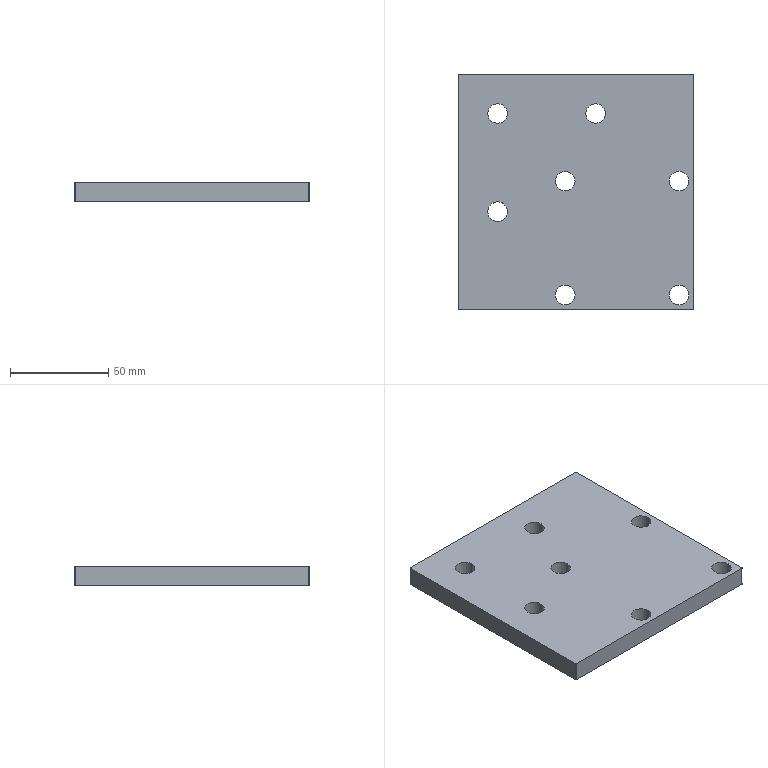Part | STEP file | Pad plate- | 1 solid | 24 faces | box 120 x 120 x 10 mm | volume 138500 mm3 | cylinder 18 | plane 6 | commonest cylinder face diameters 10 x14 1 x4
STEP:
#1=CARTESIAN_POINT('',(-392.5,287.5,10.));
#2=VERTEX_POINT('',#1);
#3=CARTESIAN_POINT('',(-382.5,287.5,10.));
#4=VERTEX_POINT('',#3);
#5=CARTESIAN_POINT('',(-387.5,287.5,10.));
#6=DIRECTION('',(0.,0.,1.));
#7=DIRECTION('',(1.,0.,0.));
#8=AXIS2_PLACEMENT_3D('',#5,#6,#7);
#9=CIRCLE('',#8,5.);
#10=EDGE_CURVE('',#2,#4,#9,.T.);
#11=ORIENTED_EDGE('',*,*,#10,.T.);
#12=CARTESIAN_POINT('',(-382.5,287.5,0.));
#13=VERTEX_POINT('',#12);
#14=CARTESIAN_POINT('',(-382.5,287.5,10.));
#15=DIRECTION('',(0.,0.,-1.));
#16=VECTOR('',#15,1000.);
#17=LINE('',#14,#16);
#18=EDGE_CURVE('',#4,#13,#17,.T.);
#19=ORIENTED_EDGE('',*,*,#18,.T.);
#20=CARTESIAN_POINT('',(-392.5,287.5,0.));
#21=VERTEX_POINT('',#20);
#22=CARTESIAN_POINT('',(-387.5,287.5,0.));
#23=DIRECTION('',(0.,0.,1.));
#24=DIRECTION('',(1.,0.,0.));
#25=AXIS2_PLACEMENT_3D('',#22,#23,#24);
#26=CIRCLE('',#25,5.);
#27=EDGE_CURVE('',#21,#13,#26,.T.);
#28=ORIENTED_EDGE('',*,*,#27,.F.);
#29=CARTESIAN_POINT('',(-392.5,287.5,10.));
#30=DIRECTION('',(0.,0.,-1.));
#31=VECTOR('',#30,1000.);
#32=LINE('',#29,#31);
#33=EDGE_CURVE('',#2,#21,#32,.T.);
#34=ORIENTED_EDGE('',*,*,#33,.F.);
#35=EDGE_LOOP('',(#11,#19,#28,#34));
#36=FACE_OUTER_BOUND('',#35,.T.);
#37=CARTESIAN_POINT('',(-387.5,287.5,10.));
#38=DIRECTION('',(0.,0.,-1.));
#39=DIRECTION('',(-1.,0.,0.));
#40=AXIS2_PLACEMENT_3D('',#37,#38,#39);
#41=CYLINDRICAL_SURFACE('',#40,5.);
#42=ADVANCED_FACE('',(#36),#41,.F.);
#43=CARTESIAN_POINT('',(-450.499,287.494,10.));
#44=VERTEX_POINT('',#43);
#45=CARTESIAN_POINT('',(-440.499,287.494,10.));
#46=VERTEX_POINT('',#45);
#47=CARTESIAN_POINT('',(-445.499,287.494,10.));
#48=DIRECTION('',(0.,0.,1.));
#49=DIRECTION('',(1.,0.,0.));
#50=AXIS2_PLACEMENT_3D('',#47,#48,#49);
#51=CIRCLE('',#50,5.);
#52=EDGE_CURVE('',#44,#46,#51,.T.);
#53=ORIENTED_EDGE('',*,*,#52,.T.);
#54=CARTESIAN_POINT('',(-440.499,287.494,0.));
#55=VERTEX_POINT('',#54);
#56=CARTESIAN_POINT('',(-440.499,287.494,10.));
#57=DIRECTION('',(0.,0.,-1.));
#58=VECTOR('',#57,1000.);
#59=LINE('',#56,#58);
#60=EDGE_CURVE('',#46,#55,#59,.T.);
#61=ORIENTED_EDGE('',*,*,#60,.T.);
#62=CARTESIAN_POINT('',(-450.499,287.494,0.));
#63=VERTEX_POINT('',#62);
#64=CARTESIAN_POINT('',(-445.499,287.494,0.));
#65=DIRECTION('',(0.,0.,1.));
#66=DIRECTION('',(1.,0.,0.));
#67=AXIS2_PLACEMENT_3D('',#64,#65,#66);
#68=CIRCLE('',#67,5.);
#69=EDGE_CURVE('',#63,#55,#68,.T.);
#70=ORIENTED_EDGE('',*,*,#69,.F.);
#71=CARTESIAN_POINT('',(-450.499,287.494,10.));
#72=DIRECTION('',(0.,0.,-1.));
#73=VECTOR('',#72,1000.);
#74=LINE('',#71,#73);
#75=EDGE_CURVE('',#44,#63,#74,.T.);
#76=ORIENTED_EDGE('',*,*,#75,.F.);
#77=EDGE_LOOP('',(#53,#61,#70,#76));
#78=FACE_OUTER_BOUND('',#77,.T.);
#79=CARTESIAN_POINT('',(-445.499,287.494,10.));
#80=DIRECTION('',(0.,0.,-1.));
#81=DIRECTION('',(-1.,0.,0.));
#82=AXIS2_PLACEMENT_3D('',#79,#80,#81);
#83=CYLINDRICAL_SURFACE('',#82,5.);
#84=ADVANCED_FACE('',(#78),#83,.F.);
#85=CARTESIAN_POINT('',(-392.5,345.5,10.));
#86=VERTEX_POINT('',#85);
#87=CARTESIAN_POINT('',(-382.5,345.5,10.));
#88=VERTEX_POINT('',#87);
#89=CARTESIAN_POINT('',(-387.5,345.5,10.));
#90=DIRECTION('',(0.,0.,1.));
#91=DIRECTION('',(1.,0.,0.));
#92=AXIS2_PLACEMENT_3D('',#89,#90,#91);
#93=CIRCLE('',#92,5.);
#94=EDGE_CURVE('',#86,#88,#93,.T.);
#95=ORIENTED_EDGE('',*,*,#94,.T.);
#96=CARTESIAN_POINT('',(-382.5,345.5,0.));
#97=VERTEX_POINT('',#96);
#98=CARTESIAN_POINT('',(-382.5,345.5,10.));
#99=DIRECTION('',(0.,0.,-1.));
#100=VECTOR('',#99,1000.);
#101=LINE('',#98,#100);
#102=EDGE_CURVE('',#88,#97,#101,.T.);
#103=ORIENTED_EDGE('',*,*,#102,.T.);
#104=CARTESIAN_POINT('',(-392.5,345.5,0.));
#105=VERTEX_POINT('',#104);
#106=CARTESIAN_POINT('',(-387.5,345.5,0.));
#107=DIRECTION('',(0.,0.,1.));
#108=DIRECTION('',(1.,0.,0.));
#109=AXIS2_PLACEMENT_3D('',#106,#107,#108);
#110=CIRCLE('',#109,5.);
#111=EDGE_CURVE('',#105,#97,#110,.T.);
#112=ORIENTED_EDGE('',*,*,#111,.F.);
#113=CARTESIAN_POINT('',(-392.5,345.5,10.));
#114=DIRECTION('',(0.,0.,-1.));
#115=VECTOR('',#114,1000.);
#116=LINE('',#113,#115);
#117=EDGE_CURVE('',#86,#105,#116,.T.);
#118=ORIENTED_EDGE('',*,*,#117,.F.);
#119=EDGE_LOOP('',(#95,#103,#112,#118));
#120=FACE_OUTER_BOUND('',#119,.T.);
#121=CARTESIAN_POINT('',(-387.5,345.5,10.));
#122=DIRECTION('',(0.,0.,-1.));
#123=DIRECTION('',(-1.,0.,0.));
#124=AXIS2_PLACEMENT_3D('',#121,#122,#123);
#125=CYLINDRICAL_SURFACE('',#124,5.);
#126=ADVANCED_FACE('',(#120),#125,.F.);
#127=CARTESIAN_POINT('',(-450.494,345.498,10.));
#128=VERTEX_POINT('',#127);
#129=CARTESIAN_POINT('',(-440.494,345.498,10.));
#130=VERTEX_POINT('',#129);
#131=CARTESIAN_POINT('',(-445.494,345.498,10.));
#132=DIRECTION('',(0.,0.,1.));
#133=DIRECTION('',(1.,0.,0.));
#134=AXIS2_PLACEMENT_3D('',#131,#132,#133);
#135=CIRCLE('',#134,5.);
#136=EDGE_CURVE('',#128,#130,#135,.T.);
#137=ORIENTED_EDGE('',*,*,#136,.T.);
#138=CARTESIAN_POINT('',(-440.494,345.498,0.));
#139=VERTEX_POINT('',#138);
#140=CARTESIAN_POINT('',(-440.494,345.498,10.));
#141=DIRECTION('',(0.,0.,-1.));
#142=VECTOR('',#141,1000.);
#143=LINE('',#140,#142);
#144=EDGE_CURVE('',#130,#139,#143,.T.);
#145=ORIENTED_EDGE('',*,*,#144,.T.);
#146=CARTESIAN_POINT('',(-450.494,345.498,0.));
#147=VERTEX_POINT('',#146);
#148=CARTESIAN_POINT('',(-445.494,345.498,0.));
#149=DIRECTION('',(0.,0.,1.));
#150=DIRECTION('',(1.,0.,0.));
#151=AXIS2_PLACEMENT_3D('',#148,#149,#150);
#152=CIRCLE('',#151,5.);
#153=EDGE_CURVE('',#147,#139,#152,.T.);
#154=ORIENTED_EDGE('',*,*,#153,.F.);
#155=CARTESIAN_POINT('',(-450.494,345.498,10.));
#156=DIRECTION('',(0.,0.,-1.));
#157=VECTOR('',#156,1000.);
#158=LINE('',#155,#157);
#159=EDGE_CURVE('',#128,#147,#158,.T.);
#160=ORIENTED_EDGE('',*,*,#159,.F.);
#161=EDGE_LOOP('',(#137,#145,#154,#160));
#162=FACE_OUTER_BOUND('',#161,.T.);
#163=CARTESIAN_POINT('',(-445.494,345.498,10.));
#164=DIRECTION('',(0.,0.,-1.));
#165=DIRECTION('',(-1.,0.,0.));
#166=AXIS2_PLACEMENT_3D('',#163,#164,#165);
#167=CYLINDRICAL_SURFACE('',#166,5.);
#168=ADVANCED_FACE('',(#162),#167,.F.);
#169=CARTESIAN_POINT('',(-485.,330.,10.));
#170=VERTEX_POINT('',#169);
#171=CARTESIAN_POINT('',(-475.,330.,10.));
#172=VERTEX_POINT('',#171);
#173=CARTESIAN_POINT('',(-480.,330.,10.));
#174=DIRECTION('',(0.,0.,1.));
#175=DIRECTION('',(1.,0.,0.));
#176=AXIS2_PLACEMENT_3D('',#173,#174,#175);
#177=CIRCLE('',#176,5.);
#178=EDGE_CURVE('',#170,#172,#177,.T.);
#179=ORIENTED_EDGE('',*,*,#178,.T.);
#180=CARTESIAN_POINT('',(-475.,330.,0.));
#181=VERTEX_POINT('',#180);
#182=CARTESIAN_POINT('',(-475.,330.,10.));
#183=DIRECTION('',(0.,0.,-1.));
#184=VECTOR('',#183,1000.);
#185=LINE('',#182,#184);
#186=EDGE_CURVE('',#172,#181,#185,.T.);
#187=ORIENTED_EDGE('',*,*,#186,.T.);
#188=CARTESIAN_POINT('',(-485.,330.,0.));
#189=VERTEX_POINT('',#188);
#190=CARTESIAN_POINT('',(-480.,330.,0.));
#191=DIRECTION('',(0.,0.,1.));
#192=DIRECTION('',(1.,0.,0.));
#193=AXIS2_PLACEMENT_3D('',#190,#191,#192);
#194=CIRCLE('',#193,5.);
#195=EDGE_CURVE('',#189,#181,#194,.T.);
#196=ORIENTED_EDGE('',*,*,#195,.F.);
#197=CARTESIAN_POINT('',(-485.,330.,10.));
#198=DIRECTION('',(0.,0.,-1.));
#199=VECTOR('',#198,1000.);
#200=LINE('',#197,#199);
#201=EDGE_CURVE('',#170,#189,#200,.T.);
#202=ORIENTED_EDGE('',*,*,#201,.F.);
#203=EDGE_LOOP('',(#179,#187,#196,#202));
#204=FACE_OUTER_BOUND('',#203,.T.);
#205=CARTESIAN_POINT('',(-480.,330.,10.));
#206=DIRECTION('',(0.,0.,-1.));
#207=DIRECTION('',(-1.,0.,0.));
#208=AXIS2_PLACEMENT_3D('',#205,#206,#207);
#209=CYLINDRICAL_SURFACE('',#208,5.);
#210=ADVANCED_FACE('',(#204),#209,.F.);
#211=CARTESIAN_POINT('',(-435.,380.,10.));
#212=VERTEX_POINT('',#211);
#213=CARTESIAN_POINT('',(-425.,380.,10.));
#214=VERTEX_POINT('',#213);
#215=CARTESIAN_POINT('',(-430.,380.,10.));
#216=DIRECTION('',(0.,0.,1.));
#217=DIRECTION('',(1.,0.,0.));
#218=AXIS2_PLACEMENT_3D('',#215,#216,#217);
#219=CIRCLE('',#218,5.);
#220=EDGE_CURVE('',#212,#214,#219,.T.);
#221=ORIENTED_EDGE('',*,*,#220,.T.);
#222=CARTESIAN_POINT('',(-425.,380.,0.));
#223=VERTEX_POINT('',#222);
#224=CARTESIAN_POINT('',(-425.,380.,10.));
#225=DIRECTION('',(0.,0.,-1.));
#226=VECTOR('',#225,1000.);
#227=LINE('',#224,#226);
#228=EDGE_CURVE('',#214,#223,#227,.T.);
#229=ORIENTED_EDGE('',*,*,#228,.T.);
#230=CARTESIAN_POINT('',(-435.,380.,0.));
#231=VERTEX_POINT('',#230);
#232=CARTESIAN_POINT('',(-430.,380.,0.));
#233=DIRECTION('',(0.,0.,1.));
#234=DIRECTION('',(1.,0.,0.));
#235=AXIS2_PLACEMENT_3D('',#232,#233,#234);
#236=CIRCLE('',#235,5.);
#237=EDGE_CURVE('',#231,#223,#236,.T.);
#238=ORIENTED_EDGE('',*,*,#237,.F.);
#239=CARTESIAN_POINT('',(-435.,380.,10.));
#240=DIRECTION('',(0.,0.,-1.));
#241=VECTOR('',#240,1000.);
#242=LINE('',#239,#241);
#243=EDGE_CURVE('',#212,#231,#242,.T.);
#244=ORIENTED_EDGE('',*,*,#243,.F.);
#245=EDGE_LOOP('',(#221,#229,#238,#244));
#246=FACE_OUTER_BOUND('',#245,.T.);
#247=CARTESIAN_POINT('',(-430.,380.,10.));
#248=DIRECTION('',(0.,0.,-1.));
#249=DIRECTION('',(-1.,0.,0.));
#250=AXIS2_PLACEMENT_3D('',#247,#248,#249);
#251=CYLINDRICAL_SURFACE('',#250,5.);
#252=ADVANCED_FACE('',(#246),#251,.F.);
#253=CARTESIAN_POINT('',(-485.,380.,10.));
#254=VERTEX_POINT('',#253);
#255=CARTESIAN_POINT('',(-475.,380.,10.));
#256=VERTEX_POINT('',#255);
#257=CARTESIAN_POINT('',(-480.,380.,10.));
#258=DIRECTION('',(0.,0.,1.));
#259=DIRECTION('',(1.,0.,0.));
#260=AXIS2_PLACEMENT_3D('',#257,#258,#259);
#261=CIRCLE('',#260,5.);
#262=EDGE_CURVE('',#254,#256,#261,.T.);
#263=ORIENTED_EDGE('',*,*,#262,.T.);
#264=CARTESIAN_POINT('',(-475.,380.,0.));
#265=VERTEX_POINT('',#264);
#266=CARTESIAN_POINT('',(-475.,380.,10.));
#267=DIRECTION('',(0.,0.,-1.));
#268=VECTOR('',#267,1000.);
#269=LINE('',#266,#268);
#270=EDGE_CURVE('',#256,#265,#269,.T.);
#271=ORIENTED_EDGE('',*,*,#270,.T.);
#272=CARTESIAN_POINT('',(-485.,380.,0.));
#273=VERTEX_POINT('',#272);
#274=CARTESIAN_POINT('',(-480.,380.,0.));
#275=DIRECTION('',(0.,0.,1.));
#276=DIRECTION('',(1.,0.,0.));
#277=AXIS2_PLACEMENT_3D('',#274,#275,#276);
#278=CIRCLE('',#277,5.);
#279=EDGE_CURVE('',#273,#265,#278,.T.);
#280=ORIENTED_EDGE('',*,*,#279,.F.);
#281=CARTESIAN_POINT('',(-485.,380.,10.));
#282=DIRECTION('',(0.,0.,-1.));
#283=VECTOR('',#282,1000.);
#284=LINE('',#281,#283);
#285=EDGE_CURVE('',#254,#273,#284,.T.);
#286=ORIENTED_EDGE('',*,*,#285,.F.);
#287=EDGE_LOOP('',(#263,#271,#280,#286));
#288=FACE_OUTER_BOUND('',#287,.T.);
#289=CARTESIAN_POINT('',(-480.,380.,10.));
#290=DIRECTION('',(0.,0.,-1.));
#291=DIRECTION('',(-1.,0.,0.));
#292=AXIS2_PLACEMENT_3D('',#289,#290,#291);
#293=CYLINDRICAL_SURFACE('',#292,5.);
#294=ADVANCED_FACE('',(#288),#293,.F.);
#295=ORIENTED_EDGE('',*,*,#52,.F.);
#296=CARTESIAN_POINT('',(-445.499,287.494,10.));
#297=DIRECTION('',(0.,0.,1.));
#298=DIRECTION('',(1.,0.,0.));
#299=AXIS2_PLACEMENT_3D('',#296,#297,#298);
#300=CIRCLE('',#299,5.);
#301=EDGE_CURVE('',#46,#44,#300,.T.);
#302=ORIENTED_EDGE('',*,*,#301,.F.);
#303=EDGE_LOOP('',(#295,#302));
#304=FACE_BOUND('',#303,.T.);
#305=ORIENTED_EDGE('',*,*,#136,.F.);
#306=CARTESIAN_POINT('',(-445.494,345.498,10.));
#307=DIRECTION('',(0.,0.,1.));
#308=DIRECTION('',(1.,0.,0.));
#309=AXIS2_PLACEMENT_3D('',#306,#307,#308);
#310=CIRCLE('',#309,5.);
#311=EDGE_CURVE('',#130,#128,#310,.T.);
#312=ORIENTED_EDGE('',*,*,#311,.F.);
#313=EDGE_LOOP('',(#305,#312));
#314=FACE_BOUND('',#313,.T.);
#315=ORIENTED_EDGE('',*,*,#220,.F.);
#316=CARTESIAN_POINT('',(-430.,380.,10.));
#317=DIRECTION('',(0.,0.,1.));
#318=DIRECTION('',(1.,0.,0.));
#319=AXIS2_PLACEMENT_3D('',#316,#317,#318);
#320=CIRCLE('',#319,5.);
#321=EDGE_CURVE('',#214,#212,#320,.T.);
#322=ORIENTED_EDGE('',*,*,#321,.F.);
#323=EDGE_LOOP('',(#315,#322));
#324=FACE_BOUND('',#323,.T.);
#325=CARTESIAN_POINT('',(-500.,399.5,10.));
#326=VERTEX_POINT('',#325);
#327=CARTESIAN_POINT('',(-500.,280.5,10.));
#328=VERTEX_POINT('',#327);
#329=CARTESIAN_POINT('',(-500.,400.,10.));
#330=DIRECTION('',(0.,-1.,0.));
#331=VECTOR('',#330,1000.);
#332=LINE('',#329,#331);
#333=EDGE_CURVE('',#326,#328,#332,.T.);
#334=ORIENTED_EDGE('',*,*,#333,.T.);
#335=CARTESIAN_POINT('',(-499.5,280.,10.));
#336=VERTEX_POINT('',#335);
#337=CARTESIAN_POINT('',(-499.5,280.5,10.));
#338=DIRECTION('',(0.,0.,1.));
#339=DIRECTION('',(1.,0.,0.));
#340=AXIS2_PLACEMENT_3D('',#337,#338,#339);
#341=CIRCLE('',#340,0.5);
#342=EDGE_CURVE('',#328,#336,#341,.T.);
#343=ORIENTED_EDGE('',*,*,#342,.T.);
#344=CARTESIAN_POINT('',(-380.5,280.,10.));
#345=VERTEX_POINT('',#344);
#346=CARTESIAN_POINT('',(-500.,280.,10.));
#347=DIRECTION('',(1.,0.,0.));
#348=VECTOR('',#347,1000.);
#349=LINE('',#346,#348);
#350=EDGE_CURVE('',#336,#345,#349,.T.);
#351=ORIENTED_EDGE('',*,*,#350,.T.);
#352=CARTESIAN_POINT('',(-380.,280.5,10.));
#353=VERTEX_POINT('',#352);
#354=CARTESIAN_POINT('',(-380.5,280.5,10.));
#355=DIRECTION('',(0.,0.,1.));
#356=DIRECTION('',(1.,0.,0.));
#357=AXIS2_PLACEMENT_3D('',#354,#355,#356);
#358=CIRCLE('',#357,0.5);
#359=EDGE_CURVE('',#345,#353,#358,.T.);
#360=ORIENTED_EDGE('',*,*,#359,.T.);
#361=CARTESIAN_POINT('',(-380.,399.5,10.));
#362=VERTEX_POINT('',#361);
#363=CARTESIAN_POINT('',(-380.,400.,10.));
#364=DIRECTION('',(0.,1.,0.));
#365=VECTOR('',#364,1000.);
#366=LINE('',#363,#365);
#367=EDGE_CURVE('',#353,#362,#366,.T.);
#368=ORIENTED_EDGE('',*,*,#367,.T.);
#369=CARTESIAN_POINT('',(-380.5,400.,10.));
#370=VERTEX_POINT('',#369);
#371=CARTESIAN_POINT('',(-380.5,399.5,10.));
#372=DIRECTION('',(0.,0.,1.));
#373=DIRECTION('',(1.,0.,0.));
#374=AXIS2_PLACEMENT_3D('',#371,#372,#373);
#375=CIRCLE('',#374,0.5);
#376=EDGE_CURVE('',#362,#370,#375,.T.);
#377=ORIENTED_EDGE('',*,*,#376,.T.);
#378=CARTESIAN_POINT('',(-499.5,400.,10.));
#379=VERTEX_POINT('',#378);
#380=CARTESIAN_POINT('',(-500.,400.,10.));
#381=DIRECTION('',(-1.,0.,0.));
#382=VECTOR('',#381,1000.);
#383=LINE('',#380,#382);
#384=EDGE_CURVE('',#370,#379,#383,.T.);
#385=ORIENTED_EDGE('',*,*,#384,.T.);
#386=CARTESIAN_POINT('',(-499.5,399.5,10.));
#387=DIRECTION('',(0.,0.,1.));
#388=DIRECTION('',(1.,0.,0.));
#389=AXIS2_PLACEMENT_3D('',#386,#387,#388);
#390=CIRCLE('',#389,0.5);
#391=EDGE_CURVE('',#379,#326,#390,.T.);
#392=ORIENTED_EDGE('',*,*,#391,.T.);
#393=EDGE_LOOP('',(#334,#343,#351,#360,#368,#377,#385,#392));
#394=FACE_OUTER_BOUND('',#393,.T.);
#395=ORIENTED_EDGE('',*,*,#262,.F.);
#396=CARTESIAN_POINT('',(-480.,380.,10.));
#397=DIRECTION('',(0.,0.,1.));
#398=DIRECTION('',(1.,0.,0.));
#399=AXIS2_PLACEMENT_3D('',#396,#397,#398);
#400=CIRCLE('',#399,5.);
#401=EDGE_CURVE('',#256,#254,#400,.T.);
#402=ORIENTED_EDGE('',*,*,#401,.F.);
#403=EDGE_LOOP('',(#395,#402));
#404=FACE_BOUND('',#403,.T.);
#405=ORIENTED_EDGE('',*,*,#178,.F.);
#406=CARTESIAN_POINT('',(-480.,330.,10.));
#407=DIRECTION('',(0.,0.,1.));
#408=DIRECTION('',(1.,0.,0.));
#409=AXIS2_PLACEMENT_3D('',#406,#407,#408);
#410=CIRCLE('',#409,5.);
#411=EDGE_CURVE('',#172,#170,#410,.T.);
#412=ORIENTED_EDGE('',*,*,#411,.F.);
#413=EDGE_LOOP('',(#405,#412));
#414=FACE_BOUND('',#413,.T.);
#415=ORIENTED_EDGE('',*,*,#94,.F.);
#416=CARTESIAN_POINT('',(-387.5,345.5,10.));
#417=DIRECTION('',(0.,0.,1.));
#418=DIRECTION('',(1.,0.,0.));
#419=AXIS2_PLACEMENT_3D('',#416,#417,#418);
#420=CIRCLE('',#419,5.);
#421=EDGE_CURVE('',#88,#86,#420,.T.);
#422=ORIENTED_EDGE('',*,*,#421,.F.);
#423=EDGE_LOOP('',(#415,#422));
#424=FACE_BOUND('',#423,.T.);
#425=ORIENTED_EDGE('',*,*,#10,.F.);
#426=CARTESIAN_POINT('',(-387.5,287.5,10.));
#427=DIRECTION('',(0.,0.,1.));
#428=DIRECTION('',(1.,0.,0.));
#429=AXIS2_PLACEMENT_3D('',#426,#427,#428);
#430=CIRCLE('',#429,5.);
#431=EDGE_CURVE('',#4,#2,#430,.T.);
#432=ORIENTED_EDGE('',*,*,#431,.F.);
#433=EDGE_LOOP('',(#425,#432));
#434=FACE_BOUND('',#433,.T.);
#435=CARTESIAN_POINT('',(0.,0.,10.));
#436=DIRECTION('',(0.,0.,1.));
#437=DIRECTION('',(1.,0.,0.));
#438=AXIS2_PLACEMENT_3D('',#435,#436,#437);
#439=PLANE('',#438);
#440=ADVANCED_FACE('',(#304,#314,#324,#394,#404,#414,#424,#434),#439,.T.);
#441=CARTESIAN_POINT('',(-499.5,280.,0.));
#442=VERTEX_POINT('',#441);
#443=CARTESIAN_POINT('',(-380.5,280.,0.));
#444=VERTEX_POINT('',#443);
#445=CARTESIAN_POINT('',(-500.,280.,0.));
#446=DIRECTION('',(1.,0.,0.));
#447=VECTOR('',#446,1000.);
#448=LINE('',#445,#447);
#449=EDGE_CURVE('',#442,#444,#448,.T.);
#450=ORIENTED_EDGE('',*,*,#449,.F.);
#451=CARTESIAN_POINT('',(-500.,280.5,0.));
#452=VERTEX_POINT('',#451);
#453=CARTESIAN_POINT('',(-499.5,280.5,0.));
#454=DIRECTION('',(0.,0.,-1.));
#455=DIRECTION('',(1.,0.,0.));
#456=AXIS2_PLACEMENT_3D('',#453,#454,#455);
#457=CIRCLE('',#456,0.5);
#458=EDGE_CURVE('',#442,#452,#457,.T.);
#459=ORIENTED_EDGE('',*,*,#458,.T.);
#460=CARTESIAN_POINT('',(-500.,399.5,0.));
#461=VERTEX_POINT('',#460);
#462=CARTESIAN_POINT('',(-500.,400.,0.));
#463=DIRECTION('',(0.,-1.,0.));
#464=VECTOR('',#463,1000.);
#465=LINE('',#462,#464);
#466=EDGE_CURVE('',#461,#452,#465,.T.);
#467=ORIENTED_EDGE('',*,*,#466,.F.);
#468=CARTESIAN_POINT('',(-499.5,400.,0.));
#469=VERTEX_POINT('',#468);
#470=CARTESIAN_POINT('',(-499.5,399.5,0.));
#471=DIRECTION('',(0.,0.,-1.));
#472=DIRECTION('',(1.,0.,0.));
#473=AXIS2_PLACEMENT_3D('',#470,#471,#472);
#474=CIRCLE('',#473,0.5);
#475=EDGE_CURVE('',#461,#469,#474,.T.);
#476=ORIENTED_EDGE('',*,*,#475,.T.);
#477=CARTESIAN_POINT('',(-380.5,400.,0.));
#478=VERTEX_POINT('',#477);
#479=CARTESIAN_POINT('',(-500.,400.,0.));
#480=DIRECTION('',(-1.,0.,0.));
#481=VECTOR('',#480,1000.);
#482=LINE('',#479,#481);
#483=EDGE_CURVE('',#478,#469,#482,.T.);
#484=ORIENTED_EDGE('',*,*,#483,.F.);
#485=CARTESIAN_POINT('',(-380.,399.5,0.));
#486=VERTEX_POINT('',#485);
#487=CARTESIAN_POINT('',(-380.5,399.5,0.));
#488=DIRECTION('',(0.,0.,-1.));
#489=DIRECTION('',(1.,0.,0.));
#490=AXIS2_PLACEMENT_3D('',#487,#488,#489);
#491=CIRCLE('',#490,0.5);
#492=EDGE_CURVE('',#478,#486,#491,.T.);
#493=ORIENTED_EDGE('',*,*,#492,.T.);
#494=CARTESIAN_POINT('',(-380.,280.5,0.));
#495=VERTEX_POINT('',#494);
#496=CARTESIAN_POINT('',(-380.,400.,0.));
#497=DIRECTION('',(0.,1.,0.));
#498=VECTOR('',#497,1000.);
#499=LINE('',#496,#498);
#500=EDGE_CURVE('',#495,#486,#499,.T.);
#501=ORIENTED_EDGE('',*,*,#500,.F.);
#502=CARTESIAN_POINT('',(-380.5,280.5,0.));
#503=DIRECTION('',(0.,0.,-1.));
#504=DIRECTION('',(1.,0.,0.));
#505=AXIS2_PLACEMENT_3D('',#502,#503,#504);
#506=CIRCLE('',#505,0.5);
#507=EDGE_CURVE('',#495,#444,#506,.T.);
#508=ORIENTED_EDGE('',*,*,#507,.T.);
#509=EDGE_LOOP('',(#450,#459,#467,#476,#484,#493,#501,#508));
#510=FACE_OUTER_BOUND('',#509,.T.);
#511=ORIENTED_EDGE('',*,*,#279,.T.);
#512=CARTESIAN_POINT('',(-480.,380.,0.));
#513=DIRECTION('',(0.,0.,1.));
#514=DIRECTION('',(1.,0.,0.));
#515=AXIS2_PLACEMENT_3D('',#512,#513,#514);
#516=CIRCLE('',#515,5.);
#517=EDGE_CURVE('',#265,#273,#516,.T.);
#518=ORIENTED_EDGE('',*,*,#517,.T.);
#519=EDGE_LOOP('',(#511,#518));
#520=FACE_BOUND('',#519,.T.);
#521=ORIENTED_EDGE('',*,*,#237,.T.);
#522=CARTESIAN_POINT('',(-430.,380.,0.));
#523=DIRECTION('',(0.,0.,1.));
#524=DIRECTION('',(1.,0.,0.));
#525=AXIS2_PLACEMENT_3D('',#522,#523,#524);
#526=CIRCLE('',#525,5.);
#527=EDGE_CURVE('',#223,#231,#526,.T.);
#528=ORIENTED_EDGE('',*,*,#527,.T.);
#529=EDGE_LOOP('',(#521,#528));
#530=FACE_BOUND('',#529,.T.);
#531=ORIENTED_EDGE('',*,*,#195,.T.);
#532=CARTESIAN_POINT('',(-480.,330.,0.));
#533=DIRECTION('',(0.,0.,1.));
#534=DIRECTION('',(1.,0.,0.));
#535=AXIS2_PLACEMENT_3D('',#532,#533,#534);
#536=CIRCLE('',#535,5.);
#537=EDGE_CURVE('',#181,#189,#536,.T.);
#538=ORIENTED_EDGE('',*,*,#537,.T.);
#539=EDGE_LOOP('',(#531,#538));
#540=FACE_BOUND('',#539,.T.);
#541=ORIENTED_EDGE('',*,*,#153,.T.);
#542=CARTESIAN_POINT('',(-445.494,345.498,0.));
#543=DIRECTION('',(0.,0.,1.));
#544=DIRECTION('',(1.,0.,0.));
#545=AXIS2_PLACEMENT_3D('',#542,#543,#544);
#546=CIRCLE('',#545,5.);
#547=EDGE_CURVE('',#139,#147,#546,.T.);
#548=ORIENTED_EDGE('',*,*,#547,.T.);
#549=EDGE_LOOP('',(#541,#548));
#550=FACE_BOUND('',#549,.T.);
#551=ORIENTED_EDGE('',*,*,#111,.T.);
#552=CARTESIAN_POINT('',(-387.5,345.5,0.));
#553=DIRECTION('',(0.,0.,1.));
#554=DIRECTION('',(1.,0.,0.));
#555=AXIS2_PLACEMENT_3D('',#552,#553,#554);
#556=CIRCLE('',#555,5.);
#557=EDGE_CURVE('',#97,#105,#556,.T.);
#558=ORIENTED_EDGE('',*,*,#557,.T.);
#559=EDGE_LOOP('',(#551,#558));
#560=FACE_BOUND('',#559,.T.);
#561=ORIENTED_EDGE('',*,*,#69,.T.);
#562=CARTESIAN_POINT('',(-445.499,287.494,0.));
#563=DIRECTION('',(0.,0.,1.));
#564=DIRECTION('',(1.,0.,0.));
#565=AXIS2_PLACEMENT_3D('',#562,#563,#564);
#566=CIRCLE('',#565,5.);
#567=EDGE_CURVE('',#55,#63,#566,.T.);
#568=ORIENTED_EDGE('',*,*,#567,.T.);
#569=EDGE_LOOP('',(#561,#568));
#570=FACE_BOUND('',#569,.T.);
#571=ORIENTED_EDGE('',*,*,#27,.T.);
#572=CARTESIAN_POINT('',(-387.5,287.5,0.));
#573=DIRECTION('',(0.,0.,1.));
#574=DIRECTION('',(1.,0.,0.));
#575=AXIS2_PLACEMENT_3D('',#572,#573,#574);
#576=CIRCLE('',#575,5.);
#577=EDGE_CURVE('',#13,#21,#576,.T.);
#578=ORIENTED_EDGE('',*,*,#577,.T.);
#579=EDGE_LOOP('',(#571,#578));
#580=FACE_BOUND('',#579,.T.);
#581=CARTESIAN_POINT('',(0.,0.,0.));
#582=DIRECTION('',(0.,0.,1.));
#583=DIRECTION('',(1.,0.,0.));
#584=AXIS2_PLACEMENT_3D('',#581,#582,#583);
#585=PLANE('',#584);
#586=ADVANCED_FACE('',(#510,#520,#530,#540,#550,#560,#570,#580),#585,.F.);
#587=ORIENTED_EDGE('',*,*,#466,.T.);
#588=CARTESIAN_POINT('',(-500.,280.5,10.));
#589=DIRECTION('',(0.,0.,1.));
#590=VECTOR('',#589,1000.);
#591=LINE('',#588,#590);
#592=EDGE_CURVE('',#452,#328,#591,.T.);
#593=ORIENTED_EDGE('',*,*,#592,.T.);
#594=ORIENTED_EDGE('',*,*,#333,.F.);
#595=CARTESIAN_POINT('',(-500.,399.5,10.));
#596=DIRECTION('',(0.,0.,-1.));
#597=VECTOR('',#596,1000.);
#598=LINE('',#595,#597);
#599=EDGE_CURVE('',#326,#461,#598,.T.);
#600=ORIENTED_EDGE('',*,*,#599,.T.);
#601=EDGE_LOOP('',(#587,#593,#594,#600));
#602=FACE_OUTER_BOUND('',#601,.T.);
#603=CARTESIAN_POINT('',(-500.,400.,10.));
#604=DIRECTION('',(1.,0.,0.));
#605=DIRECTION('',(0.,0.,-1.));
#606=AXIS2_PLACEMENT_3D('',#603,#604,#605);
#607=PLANE('',#606);
#608=ADVANCED_FACE('',(#602),#607,.F.);
#609=ORIENTED_EDGE('',*,*,#350,.F.);
#610=CARTESIAN_POINT('',(-499.5,280.,10.));
#611=DIRECTION('',(0.,0.,-1.));
#612=VECTOR('',#611,1000.);
#613=LINE('',#610,#612);
#614=EDGE_CURVE('',#336,#442,#613,.T.);
#615=ORIENTED_EDGE('',*,*,#614,.T.);
#616=ORIENTED_EDGE('',*,*,#449,.T.);
#617=CARTESIAN_POINT('',(-380.5,280.,10.));
#618=DIRECTION('',(0.,0.,1.));
#619=VECTOR('',#618,1000.);
#620=LINE('',#617,#619);
#621=EDGE_CURVE('',#444,#345,#620,.T.);
#622=ORIENTED_EDGE('',*,*,#621,.T.);
#623=EDGE_LOOP('',(#609,#615,#616,#622));
#624=FACE_OUTER_BOUND('',#623,.T.);
#625=CARTESIAN_POINT('',(-500.,280.,10.));
#626=DIRECTION('',(0.,1.,0.));
#627=DIRECTION('',(0.,0.,1.));
#628=AXIS2_PLACEMENT_3D('',#625,#626,#627);
#629=PLANE('',#628);
#630=ADVANCED_FACE('',(#624),#629,.F.);
#631=ORIENTED_EDGE('',*,*,#367,.F.);
#632=CARTESIAN_POINT('',(-380.,280.5,10.));
#633=DIRECTION('',(0.,0.,-1.));
#634=VECTOR('',#633,1000.);
#635=LINE('',#632,#634);
#636=EDGE_CURVE('',#353,#495,#635,.T.);
#637=ORIENTED_EDGE('',*,*,#636,.T.);
#638=ORIENTED_EDGE('',*,*,#500,.T.);
#639=CARTESIAN_POINT('',(-380.,399.5,10.));
#640=DIRECTION('',(0.,0.,1.));
#641=VECTOR('',#640,1000.);
#642=LINE('',#639,#641);
#643=EDGE_CURVE('',#486,#362,#642,.T.);
#644=ORIENTED_EDGE('',*,*,#643,.T.);
#645=EDGE_LOOP('',(#631,#637,#638,#644));
#646=FACE_OUTER_BOUND('',#645,.T.);
#647=CARTESIAN_POINT('',(-380.,400.,10.));
#648=DIRECTION('',(-1.,0.,0.));
#649=DIRECTION('',(0.,0.,1.));
#650=AXIS2_PLACEMENT_3D('',#647,#648,#649);
#651=PLANE('',#650);
#652=ADVANCED_FACE('',(#646),#651,.F.);
#653=ORIENTED_EDGE('',*,*,#384,.F.);
#654=CARTESIAN_POINT('',(-380.5,400.,10.));
#655=DIRECTION('',(0.,0.,-1.));
#656=VECTOR('',#655,1000.);
#657=LINE('',#654,#656);
#658=EDGE_CURVE('',#370,#478,#657,.T.);
#659=ORIENTED_EDGE('',*,*,#658,.T.);
#660=ORIENTED_EDGE('',*,*,#483,.T.);
#661=CARTESIAN_POINT('',(-499.5,400.,10.));
#662=DIRECTION('',(0.,0.,1.));
#663=VECTOR('',#662,1000.);
#664=LINE('',#661,#663);
#665=EDGE_CURVE('',#469,#379,#664,.T.);
#666=ORIENTED_EDGE('',*,*,#665,.T.);
#667=EDGE_LOOP('',(#653,#659,#660,#666));
#668=FACE_OUTER_BOUND('',#667,.T.);
#669=CARTESIAN_POINT('',(-500.,400.,10.));
#670=DIRECTION('',(0.,-1.,0.));
#671=DIRECTION('',(0.,0.,-1.));
#672=AXIS2_PLACEMENT_3D('',#669,#670,#671);
#673=PLANE('',#672);
#674=ADVANCED_FACE('',(#668),#673,.F.);
#675=ORIENTED_EDGE('',*,*,#270,.F.);
#676=ORIENTED_EDGE('',*,*,#401,.T.);
#677=ORIENTED_EDGE('',*,*,#285,.T.);
#678=ORIENTED_EDGE('',*,*,#517,.F.);
#679=EDGE_LOOP('',(#675,#676,#677,#678));
#680=FACE_OUTER_BOUND('',#679,.T.);
#681=CARTESIAN_POINT('',(-480.,380.,10.));
#682=DIRECTION('',(0.,0.,-1.));
#683=DIRECTION('',(-1.,0.,0.));
#684=AXIS2_PLACEMENT_3D('',#681,#682,#683);
#685=CYLINDRICAL_SURFACE('',#684,5.);
#686=ADVANCED_FACE('',(#680),#685,.F.);
#687=ORIENTED_EDGE('',*,*,#228,.F.);
#688=ORIENTED_EDGE('',*,*,#321,.T.);
#689=ORIENTED_EDGE('',*,*,#243,.T.);
#690=ORIENTED_EDGE('',*,*,#527,.F.);
#691=EDGE_LOOP('',(#687,#688,#689,#690));
#692=FACE_OUTER_BOUND('',#691,.T.);
#693=CARTESIAN_POINT('',(-430.,380.,10.));
#694=DIRECTION('',(0.,0.,-1.));
#695=DIRECTION('',(-1.,0.,0.));
#696=AXIS2_PLACEMENT_3D('',#693,#694,#695);
#697=CYLINDRICAL_SURFACE('',#696,5.);
#698=ADVANCED_FACE('',(#692),#697,.F.);
#699=ORIENTED_EDGE('',*,*,#186,.F.);
#700=ORIENTED_EDGE('',*,*,#411,.T.);
#701=ORIENTED_EDGE('',*,*,#201,.T.);
#702=ORIENTED_EDGE('',*,*,#537,.F.);
#703=EDGE_LOOP('',(#699,#700,#701,#702));
#704=FACE_OUTER_BOUND('',#703,.T.);
#705=CARTESIAN_POINT('',(-480.,330.,10.));
#706=DIRECTION('',(0.,0.,-1.));
#707=DIRECTION('',(-1.,0.,0.));
#708=AXIS2_PLACEMENT_3D('',#705,#706,#707);
#709=CYLINDRICAL_SURFACE('',#708,5.);
#710=ADVANCED_FACE('',(#704),#709,.F.);
#711=ORIENTED_EDGE('',*,*,#144,.F.);
#712=ORIENTED_EDGE('',*,*,#311,.T.);
#713=ORIENTED_EDGE('',*,*,#159,.T.);
#714=ORIENTED_EDGE('',*,*,#547,.F.);
#715=EDGE_LOOP('',(#711,#712,#713,#714));
#716=FACE_OUTER_BOUND('',#715,.T.);
#717=CARTESIAN_POINT('',(-445.494,345.498,10.));
#718=DIRECTION('',(0.,0.,-1.));
#719=DIRECTION('',(-1.,0.,0.));
#720=AXIS2_PLACEMENT_3D('',#717,#718,#719);
#721=CYLINDRICAL_SURFACE('',#720,5.);
#722=ADVANCED_FACE('',(#716),#721,.F.);
#723=ORIENTED_EDGE('',*,*,#102,.F.);
#724=ORIENTED_EDGE('',*,*,#421,.T.);
#725=ORIENTED_EDGE('',*,*,#117,.T.);
#726=ORIENTED_EDGE('',*,*,#557,.F.);
#727=EDGE_LOOP('',(#723,#724,#725,#726));
#728=FACE_OUTER_BOUND('',#727,.T.);
#729=CARTESIAN_POINT('',(-387.5,345.5,10.));
#730=DIRECTION('',(0.,0.,-1.));
#731=DIRECTION('',(-1.,0.,0.));
#732=AXIS2_PLACEMENT_3D('',#729,#730,#731);
#733=CYLINDRICAL_SURFACE('',#732,5.);
#734=ADVANCED_FACE('',(#728),#733,.F.);
#735=ORIENTED_EDGE('',*,*,#60,.F.);
#736=ORIENTED_EDGE('',*,*,#301,.T.);
#737=ORIENTED_EDGE('',*,*,#75,.T.);
#738=ORIENTED_EDGE('',*,*,#567,.F.);
#739=EDGE_LOOP('',(#735,#736,#737,#738));
#740=FACE_OUTER_BOUND('',#739,.T.);
#741=CARTESIAN_POINT('',(-445.499,287.494,10.));
#742=DIRECTION('',(0.,0.,-1.));
#743=DIRECTION('',(-1.,0.,0.));
#744=AXIS2_PLACEMENT_3D('',#741,#742,#743);
#745=CYLINDRICAL_SURFACE('',#744,5.);
#746=ADVANCED_FACE('',(#740),#745,.F.);
#747=ORIENTED_EDGE('',*,*,#18,.F.);
#748=ORIENTED_EDGE('',*,*,#431,.T.);
#749=ORIENTED_EDGE('',*,*,#33,.T.);
#750=ORIENTED_EDGE('',*,*,#577,.F.);
#751=EDGE_LOOP('',(#747,#748,#749,#750));
#752=FACE_OUTER_BOUND('',#751,.T.);
#753=CARTESIAN_POINT('',(-387.5,287.5,10.));
#754=DIRECTION('',(0.,0.,-1.));
#755=DIRECTION('',(-1.,0.,0.));
#756=AXIS2_PLACEMENT_3D('',#753,#754,#755);
#757=CYLINDRICAL_SURFACE('',#756,5.);
#758=ADVANCED_FACE('',(#752),#757,.F.);
#759=ORIENTED_EDGE('',*,*,#342,.F.);
#760=ORIENTED_EDGE('',*,*,#592,.F.);
#761=ORIENTED_EDGE('',*,*,#458,.F.);
#762=ORIENTED_EDGE('',*,*,#614,.F.);
#763=EDGE_LOOP('',(#759,#760,#761,#762));
#764=FACE_OUTER_BOUND('',#763,.T.);
#765=CARTESIAN_POINT('',(-499.5,280.5,10.));
#766=DIRECTION('',(0.,0.,-1.));
#767=DIRECTION('',(-1.,0.,0.));
#768=AXIS2_PLACEMENT_3D('',#765,#766,#767);
#769=CYLINDRICAL_SURFACE('',#768,0.5);
#770=ADVANCED_FACE('',(#764),#769,.T.);
#771=ORIENTED_EDGE('',*,*,#359,.F.);
#772=ORIENTED_EDGE('',*,*,#621,.F.);
#773=ORIENTED_EDGE('',*,*,#507,.F.);
#774=ORIENTED_EDGE('',*,*,#636,.F.);
#775=EDGE_LOOP('',(#771,#772,#773,#774));
#776=FACE_OUTER_BOUND('',#775,.T.);
#777=CARTESIAN_POINT('',(-380.5,280.5,10.));
#778=DIRECTION('',(0.,0.,-1.));
#779=DIRECTION('',(-1.,0.,0.));
#780=AXIS2_PLACEMENT_3D('',#777,#778,#779);
#781=CYLINDRICAL_SURFACE('',#780,0.5);
#782=ADVANCED_FACE('',(#776),#781,.T.);
#783=ORIENTED_EDGE('',*,*,#376,.F.);
#784=ORIENTED_EDGE('',*,*,#643,.F.);
#785=ORIENTED_EDGE('',*,*,#492,.F.);
#786=ORIENTED_EDGE('',*,*,#658,.F.);
#787=EDGE_LOOP('',(#783,#784,#785,#786));
#788=FACE_OUTER_BOUND('',#787,.T.);
#789=CARTESIAN_POINT('',(-380.5,399.5,10.));
#790=DIRECTION('',(0.,0.,-1.));
#791=DIRECTION('',(-1.,0.,0.));
#792=AXIS2_PLACEMENT_3D('',#789,#790,#791);
#793=CYLINDRICAL_SURFACE('',#792,0.5);
#794=ADVANCED_FACE('',(#788),#793,.T.);
#795=ORIENTED_EDGE('',*,*,#391,.F.);
#796=ORIENTED_EDGE('',*,*,#665,.F.);
#797=ORIENTED_EDGE('',*,*,#475,.F.);
#798=ORIENTED_EDGE('',*,*,#599,.F.);
#799=EDGE_LOOP('',(#795,#796,#797,#798));
#800=FACE_OUTER_BOUND('',#799,.T.);
#801=CARTESIAN_POINT('',(-499.5,399.5,10.));
#802=DIRECTION('',(0.,0.,-1.));
#803=DIRECTION('',(-1.,0.,0.));
#804=AXIS2_PLACEMENT_3D('',#801,#802,#803);
#805=CYLINDRICAL_SURFACE('',#804,0.5);
#806=ADVANCED_FACE('',(#800),#805,.T.);
#807=CLOSED_SHELL('',(#42,#84,#126,#168,#210,#252,#294,#440,#586,#608,#630,#652,#674,#686,#698,#710,#722,#734,#746,#758,#770,#782,#794,#806));
#808=MANIFOLD_SOLID_BREP('',#807);
#809=CARTESIAN_POINT('',(0.,0.,0.));
#810=DIRECTION('',(0.,0.,1.));
#811=DIRECTION('',(1.,0.,0.));
#812=AXIS2_PLACEMENT_3D('',#809,#810,#811);
#813=(LENGTH_UNIT()NAMED_UNIT(*)SI_UNIT(.MILLI.,.METRE.));
#814=UNCERTAINTY_MEASURE_WITH_UNIT(LENGTH_MEASURE(0.00001),#813,'','');
#815=(NAMED_UNIT(*)PLANE_ANGLE_UNIT()SI_UNIT($,.RADIAN.));
#816=(NAMED_UNIT(*)SI_UNIT($,.STERADIAN.)SOLID_ANGLE_UNIT());
#817=(GEOMETRIC_REPRESENTATION_CONTEXT(3)GLOBAL_UNCERTAINTY_ASSIGNED_CONTEXT((#814))GLOBAL_UNIT_ASSIGNED_CONTEXT((#813,#815,#816))REPRESENTATION_CONTEXT('',''));
#818=ADVANCED_BREP_SHAPE_REPRESENTATION('',(#808,#812),#817);